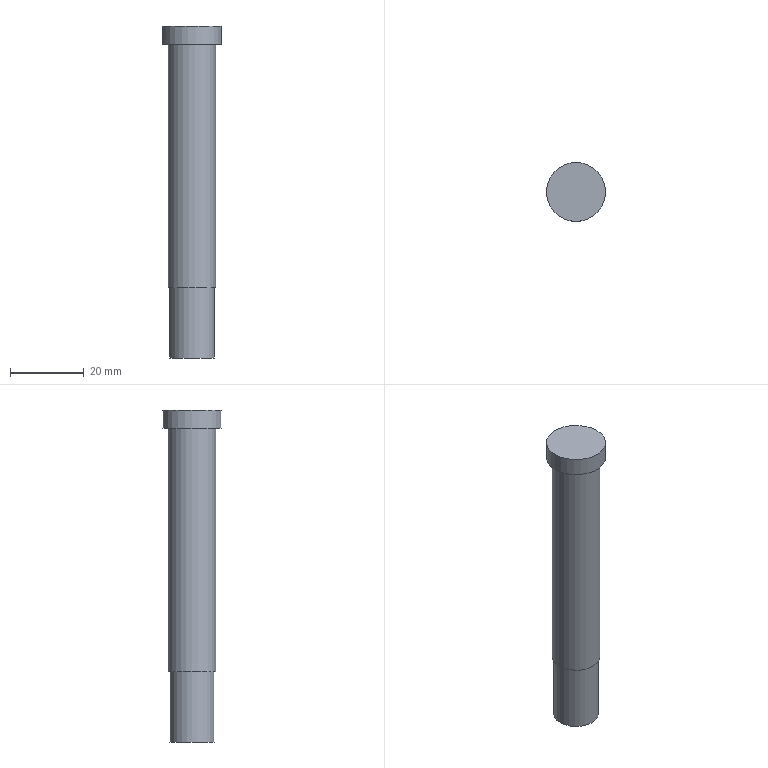Part | NX | features solid 2 | 1 solid | 7 faces | box 16 x 16 x 90 mm | volume 11950 mm3 | plane 4 | cylinder 3 | commonest cylinder face diameters 12.1 x1 13 x1 16 x1
STEP:
#1=CARTESIAN_POINT('',(259.876,-353.512,22.));
#2=VERTEX_POINT('',#1);
#3=CARTESIAN_POINT('',(253.376,-353.512,22.));
#4=DIRECTION('',(0.,0.,1.));
#5=DIRECTION('',(1.,0.,0.));
#6=AXIS2_PLACEMENT_3D('',#3,#4,#5);
#7=CIRCLE('',#6,6.5);
#8=EDGE_CURVE('',#2,#2,#7,.T.);
#9=ORIENTED_EDGE('',*,*,#8,.T.);
#10=EDGE_LOOP('',(#9));
#11=FACE_BOUND('',#10,.T.);
#12=CARTESIAN_POINT('',(259.876,-353.512,88.));
#13=VERTEX_POINT('',#12);
#14=CARTESIAN_POINT('',(253.376,-353.512,88.));
#15=DIRECTION('',(0.,0.,1.));
#16=DIRECTION('',(1.,0.,0.));
#17=AXIS2_PLACEMENT_3D('',#14,#15,#16);
#18=CIRCLE('',#17,6.5);
#19=EDGE_CURVE('',#13,#13,#18,.T.);
#20=ORIENTED_EDGE('',*,*,#19,.F.);
#21=EDGE_LOOP('',(#20));
#22=FACE_BOUND('',#21,.T.);
#23=CARTESIAN_POINT('',(253.376,-353.512,93.));
#24=DIRECTION('',(0.,0.,-1.));
#25=DIRECTION('',(-1.,0.,0.));
#26=AXIS2_PLACEMENT_3D('',#23,#24,#25);
#27=CYLINDRICAL_SURFACE('',#26,6.5);
#28=ADVANCED_FACE('',(#11,#22),#27,.T.);
#29=CARTESIAN_POINT('',(259.426,-353.512,22.));
#30=VERTEX_POINT('',#29);
#31=CARTESIAN_POINT('',(253.376,-353.512,22.));
#32=DIRECTION('',(0.,0.,1.));
#33=DIRECTION('',(1.,0.,0.));
#34=AXIS2_PLACEMENT_3D('',#31,#32,#33);
#35=CIRCLE('',#34,6.05);
#36=EDGE_CURVE('',#30,#30,#35,.T.);
#37=ORIENTED_EDGE('',*,*,#36,.T.);
#38=EDGE_LOOP('',(#37));
#39=FACE_BOUND('',#38,.T.);
#40=ORIENTED_EDGE('',*,*,#8,.F.);
#41=EDGE_LOOP('',(#40));
#42=FACE_BOUND('',#41,.T.);
#43=CARTESIAN_POINT('',(253.376,-353.512,22.));
#44=DIRECTION('',(0.,0.,1.));
#45=DIRECTION('',(1.,0.,0.));
#46=AXIS2_PLACEMENT_3D('',#43,#44,#45);
#47=PLANE('',#46);
#48=ADVANCED_FACE('',(#39,#42),#47,.F.);
#49=CARTESIAN_POINT('',(261.376,-353.512,88.));
#50=VERTEX_POINT('',#49);
#51=CARTESIAN_POINT('',(253.376,-353.512,88.));
#52=DIRECTION('',(0.,0.,1.));
#53=DIRECTION('',(1.,0.,0.));
#54=AXIS2_PLACEMENT_3D('',#51,#52,#53);
#55=CIRCLE('',#54,8.);
#56=EDGE_CURVE('',#50,#50,#55,.T.);
#57=ORIENTED_EDGE('',*,*,#56,.F.);
#58=EDGE_LOOP('',(#57));
#59=FACE_BOUND('',#58,.T.);
#60=ORIENTED_EDGE('',*,*,#19,.T.);
#61=EDGE_LOOP('',(#60));
#62=FACE_BOUND('',#61,.T.);
#63=CARTESIAN_POINT('',(253.376,-353.512,88.));
#64=DIRECTION('',(0.,0.,1.));
#65=DIRECTION('',(1.,0.,0.));
#66=AXIS2_PLACEMENT_3D('',#63,#64,#65);
#67=PLANE('',#66);
#68=ADVANCED_FACE('',(#59,#62),#67,.F.);
#69=ORIENTED_EDGE('',*,*,#56,.T.);
#70=EDGE_LOOP('',(#69));
#71=FACE_BOUND('',#70,.T.);
#72=CARTESIAN_POINT('',(261.376,-353.512,93.));
#73=VERTEX_POINT('',#72);
#74=CARTESIAN_POINT('',(253.376,-353.512,93.));
#75=DIRECTION('',(0.,0.,1.));
#76=DIRECTION('',(1.,0.,0.));
#77=AXIS2_PLACEMENT_3D('',#74,#75,#76);
#78=CIRCLE('',#77,8.);
#79=EDGE_CURVE('',#73,#73,#78,.T.);
#80=ORIENTED_EDGE('',*,*,#79,.F.);
#81=EDGE_LOOP('',(#80));
#82=FACE_BOUND('',#81,.T.);
#83=CARTESIAN_POINT('',(253.376,-353.512,88.));
#84=DIRECTION('',(0.,0.,1.));
#85=DIRECTION('',(1.,0.,0.));
#86=AXIS2_PLACEMENT_3D('',#83,#84,#85);
#87=CYLINDRICAL_SURFACE('',#86,8.);
#88=ADVANCED_FACE('',(#71,#82),#87,.T.);
#89=ORIENTED_EDGE('',*,*,#79,.T.);
#90=EDGE_LOOP('',(#89));
#91=FACE_BOUND('',#90,.T.);
#92=CARTESIAN_POINT('',(253.376,-353.512,93.));
#93=DIRECTION('',(0.,0.,1.));
#94=DIRECTION('',(1.,0.,0.));
#95=AXIS2_PLACEMENT_3D('',#92,#93,#94);
#96=PLANE('',#95);
#97=ADVANCED_FACE('',(#91),#96,.T.);
#98=CARTESIAN_POINT('',(259.426,-353.512,3.));
#99=VERTEX_POINT('',#98);
#100=CARTESIAN_POINT('',(253.376,-353.512,3.));
#101=DIRECTION('',(0.,0.,1.));
#102=DIRECTION('',(1.,0.,0.));
#103=AXIS2_PLACEMENT_3D('',#100,#101,#102);
#104=CIRCLE('',#103,6.05);
#105=EDGE_CURVE('',#99,#99,#104,.T.);
#106=ORIENTED_EDGE('',*,*,#105,.T.);
#107=EDGE_LOOP('',(#106));
#108=FACE_BOUND('',#107,.T.);
#109=ORIENTED_EDGE('',*,*,#36,.F.);
#110=EDGE_LOOP('',(#109));
#111=FACE_BOUND('',#110,.T.);
#112=CARTESIAN_POINT('',(253.376,-353.512,3.));
#113=DIRECTION('',(0.,0.,1.));
#114=DIRECTION('',(1.,0.,0.));
#115=AXIS2_PLACEMENT_3D('',#112,#113,#114);
#116=CYLINDRICAL_SURFACE('',#115,6.05);
#117=ADVANCED_FACE('',(#108,#111),#116,.T.);
#118=ORIENTED_EDGE('',*,*,#105,.F.);
#119=EDGE_LOOP('',(#118));
#120=FACE_BOUND('',#119,.T.);
#121=CARTESIAN_POINT('',(253.376,-353.512,3.));
#122=DIRECTION('',(0.,0.,1.));
#123=DIRECTION('',(1.,0.,0.));
#124=AXIS2_PLACEMENT_3D('',#121,#122,#123);
#125=PLANE('',#124);
#126=ADVANCED_FACE('',(#120),#125,.F.);
#127=CLOSED_SHELL('',(#28,#48,#68,#88,#97,#117,#126));
#128=MANIFOLD_SOLID_BREP('',#127);
#129=(LENGTH_UNIT()NAMED_UNIT(*)SI_UNIT(.MILLI.,.METRE.));
#130=UNCERTAINTY_MEASURE_WITH_UNIT(LENGTH_MEASURE(0.00001),#129,'','');
#131=(NAMED_UNIT(*)PLANE_ANGLE_UNIT()SI_UNIT($,.RADIAN.));
#132=(NAMED_UNIT(*)SI_UNIT($,.STERADIAN.)SOLID_ANGLE_UNIT());
#133=(GEOMETRIC_REPRESENTATION_CONTEXT(3)GLOBAL_UNCERTAINTY_ASSIGNED_CONTEXT((#130))GLOBAL_UNIT_ASSIGNED_CONTEXT((#129,#131,#132))REPRESENTATION_CONTEXT('',''));
#134=ADVANCED_BREP_SHAPE_REPRESENTATION('',(#128),#133);